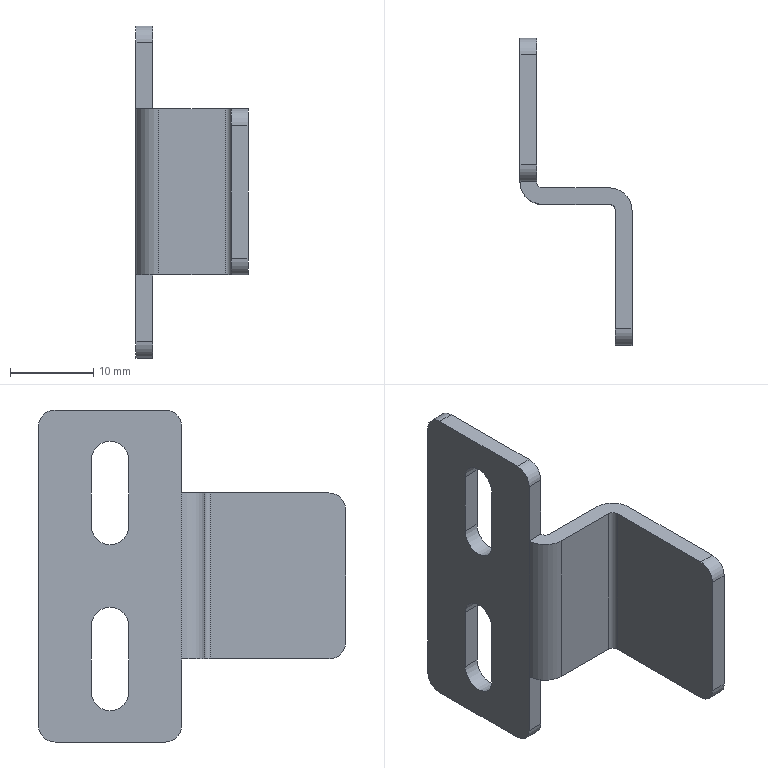Part | STEP file | 1 solid | 32 faces | box 13.5 x 37 x 40 mm | volume 2353 mm3 | plane 18 | cylinder 14 | commonest cylinder face diameters 4 x6 4.5 x4 1.473 x2 5.473 x2